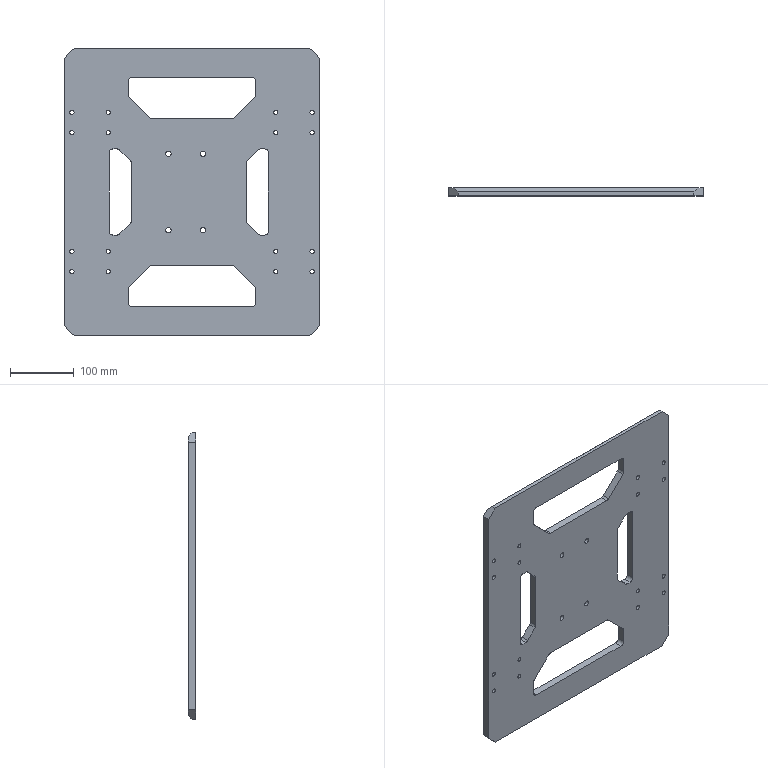Part | STEP file | PLACA BASE IZAJE | 1 solid | 100 faces | box 400 x 12 x 450 mm | volume 1745930 mm3 | cylinder 64 | plane 36 | commonest cylinder face diameters 6.8 x32 12 x24 8.5 x8